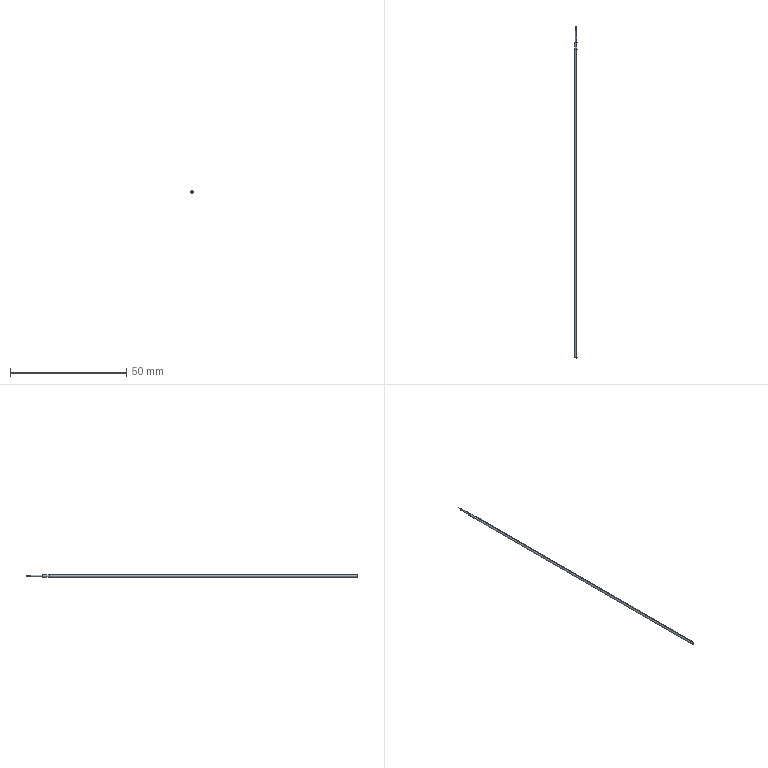Part | SolidWorks | features ICE 3, Extrusion 1 | 1 solid | 13 faces | box 1.13 x 143 x 1.13 mm | volume 137.726 mm3 | cylinder 8 | plane 5 | commonest cylinder face diameters 0.2 x2 0.7 x2 1 x2 1.13 x2
STEP:
#1=CARTESIAN_POINT('',(0.,143.,0.1));
#2=VERTEX_POINT('',#1);
#3=CARTESIAN_POINT('',(0.,143.,-0.1));
#4=VERTEX_POINT('',#3);
#5=CARTESIAN_POINT('',(0.,143.,0.));
#6=DIRECTION('',(0.,1.,0.));
#7=DIRECTION('',(0.,0.,1.));
#8=AXIS2_PLACEMENT_3D('',#5,#6,#7);
#9=CIRCLE('',#8,0.1);
#10=EDGE_CURVE('',#2,#4,#9,.T.);
#11=ORIENTED_EDGE('',*,*,#10,.F.);
#12=CARTESIAN_POINT('',(0.,141.,0.1));
#13=VERTEX_POINT('',#12);
#14=CARTESIAN_POINT('',(0.,143.,0.1));
#15=DIRECTION('',(0.,-1.,0.));
#16=VECTOR('',#15,1000.);
#17=LINE('',#14,#16);
#18=EDGE_CURVE('',#2,#13,#17,.T.);
#19=ORIENTED_EDGE('',*,*,#18,.T.);
#20=CARTESIAN_POINT('',(0.,141.,-0.1));
#21=VERTEX_POINT('',#20);
#22=CARTESIAN_POINT('',(0.,141.,0.));
#23=DIRECTION('',(0.,1.,0.));
#24=DIRECTION('',(0.,0.,1.));
#25=AXIS2_PLACEMENT_3D('',#22,#23,#24);
#26=CIRCLE('',#25,0.1);
#27=EDGE_CURVE('',#13,#21,#26,.T.);
#28=ORIENTED_EDGE('',*,*,#27,.T.);
#29=CARTESIAN_POINT('',(0.,143.,-0.1));
#30=DIRECTION('',(0.,-1.,0.));
#31=VECTOR('',#30,1000.);
#32=LINE('',#29,#31);
#33=EDGE_CURVE('',#4,#21,#32,.T.);
#34=ORIENTED_EDGE('',*,*,#33,.F.);
#35=EDGE_LOOP('',(#11,#19,#28,#34));
#36=FACE_OUTER_BOUND('',#35,.T.);
#37=CARTESIAN_POINT('',(0.,143.,0.));
#38=DIRECTION('',(0.,-1.,0.));
#39=DIRECTION('',(0.,0.,-1.));
#40=AXIS2_PLACEMENT_3D('',#37,#38,#39);
#41=CYLINDRICAL_SURFACE('',#40,0.1);
#42=ADVANCED_FACE('',(#36),#41,.T.);
#43=CARTESIAN_POINT('',(0.,141.,0.35));
#44=VERTEX_POINT('',#43);
#45=CARTESIAN_POINT('',(0.,141.,-0.35));
#46=VERTEX_POINT('',#45);
#47=CARTESIAN_POINT('',(0.,141.,0.));
#48=DIRECTION('',(0.,1.,0.));
#49=DIRECTION('',(0.,0.,1.));
#50=AXIS2_PLACEMENT_3D('',#47,#48,#49);
#51=CIRCLE('',#50,0.35);
#52=EDGE_CURVE('',#44,#46,#51,.T.);
#53=ORIENTED_EDGE('',*,*,#52,.F.);
#54=CARTESIAN_POINT('',(0.,136.,0.35));
#55=VERTEX_POINT('',#54);
#56=CARTESIAN_POINT('',(0.,141.,0.35));
#57=DIRECTION('',(0.,-1.,0.));
#58=VECTOR('',#57,1000.);
#59=LINE('',#56,#58);
#60=EDGE_CURVE('',#44,#55,#59,.T.);
#61=ORIENTED_EDGE('',*,*,#60,.T.);
#62=CARTESIAN_POINT('',(0.,136.,-0.35));
#63=VERTEX_POINT('',#62);
#64=CARTESIAN_POINT('',(0.,136.,0.));
#65=DIRECTION('',(0.,1.,0.));
#66=DIRECTION('',(0.,0.,1.));
#67=AXIS2_PLACEMENT_3D('',#64,#65,#66);
#68=CIRCLE('',#67,0.35);
#69=EDGE_CURVE('',#55,#63,#68,.T.);
#70=ORIENTED_EDGE('',*,*,#69,.T.);
#71=CARTESIAN_POINT('',(0.,141.,-0.35));
#72=DIRECTION('',(0.,-1.,0.));
#73=VECTOR('',#72,1000.);
#74=LINE('',#71,#73);
#75=EDGE_CURVE('',#46,#63,#74,.T.);
#76=ORIENTED_EDGE('',*,*,#75,.F.);
#77=EDGE_LOOP('',(#53,#61,#70,#76));
#78=FACE_OUTER_BOUND('',#77,.T.);
#79=CARTESIAN_POINT('',(0.,141.,0.));
#80=DIRECTION('',(0.,-1.,0.));
#81=DIRECTION('',(0.,0.,-1.));
#82=AXIS2_PLACEMENT_3D('',#79,#80,#81);
#83=CYLINDRICAL_SURFACE('',#82,0.35);
#84=ADVANCED_FACE('',(#78),#83,.T.);
#85=CARTESIAN_POINT('',(0.,136.,0.5));
#86=VERTEX_POINT('',#85);
#87=CARTESIAN_POINT('',(0.,136.,-0.5));
#88=VERTEX_POINT('',#87);
#89=CARTESIAN_POINT('',(0.,136.,0.));
#90=DIRECTION('',(0.,1.,0.));
#91=DIRECTION('',(0.,0.,1.));
#92=AXIS2_PLACEMENT_3D('',#89,#90,#91);
#93=CIRCLE('',#92,0.5);
#94=EDGE_CURVE('',#86,#88,#93,.T.);
#95=ORIENTED_EDGE('',*,*,#94,.F.);
#96=CARTESIAN_POINT('',(0.,133.,0.5));
#97=VERTEX_POINT('',#96);
#98=CARTESIAN_POINT('',(0.,136.,0.5));
#99=DIRECTION('',(0.,-1.,0.));
#100=VECTOR('',#99,1000.);
#101=LINE('',#98,#100);
#102=EDGE_CURVE('',#86,#97,#101,.T.);
#103=ORIENTED_EDGE('',*,*,#102,.T.);
#104=CARTESIAN_POINT('',(0.,133.,-0.5));
#105=VERTEX_POINT('',#104);
#106=CARTESIAN_POINT('',(0.,133.,0.));
#107=DIRECTION('',(0.,1.,0.));
#108=DIRECTION('',(0.,0.,1.));
#109=AXIS2_PLACEMENT_3D('',#106,#107,#108);
#110=CIRCLE('',#109,0.5);
#111=EDGE_CURVE('',#97,#105,#110,.T.);
#112=ORIENTED_EDGE('',*,*,#111,.T.);
#113=CARTESIAN_POINT('',(0.,136.,-0.5));
#114=DIRECTION('',(0.,-1.,0.));
#115=VECTOR('',#114,1000.);
#116=LINE('',#113,#115);
#117=EDGE_CURVE('',#88,#105,#116,.T.);
#118=ORIENTED_EDGE('',*,*,#117,.F.);
#119=EDGE_LOOP('',(#95,#103,#112,#118));
#120=FACE_OUTER_BOUND('',#119,.T.);
#121=CARTESIAN_POINT('',(0.,136.,0.));
#122=DIRECTION('',(0.,-1.,0.));
#123=DIRECTION('',(0.,0.,-1.));
#124=AXIS2_PLACEMENT_3D('',#121,#122,#123);
#125=CYLINDRICAL_SURFACE('',#124,0.5);
#126=ADVANCED_FACE('',(#120),#125,.T.);
#127=CARTESIAN_POINT('',(0.,133.,0.565));
#128=VERTEX_POINT('',#127);
#129=CARTESIAN_POINT('',(0.,133.,-0.565));
#130=VERTEX_POINT('',#129);
#131=CARTESIAN_POINT('',(0.,133.,0.));
#132=DIRECTION('',(0.,1.,0.));
#133=DIRECTION('',(0.,0.,1.));
#134=AXIS2_PLACEMENT_3D('',#131,#132,#133);
#135=CIRCLE('',#134,0.565);
#136=EDGE_CURVE('',#128,#130,#135,.T.);
#137=ORIENTED_EDGE('',*,*,#136,.F.);
#138=CARTESIAN_POINT('',(0.,0.,0.565));
#139=VERTEX_POINT('',#138);
#140=CARTESIAN_POINT('',(0.,133.,0.565));
#141=DIRECTION('',(0.,-1.,0.));
#142=VECTOR('',#141,1000.);
#143=LINE('',#140,#142);
#144=EDGE_CURVE('',#128,#139,#143,.T.);
#145=ORIENTED_EDGE('',*,*,#144,.T.);
#146=CARTESIAN_POINT('',(0.,0.,-0.565));
#147=VERTEX_POINT('',#146);
#148=CARTESIAN_POINT('',(0.,0.,0.));
#149=DIRECTION('',(0.,1.,0.));
#150=DIRECTION('',(0.,0.,1.));
#151=AXIS2_PLACEMENT_3D('',#148,#149,#150);
#152=CIRCLE('',#151,0.565);
#153=EDGE_CURVE('',#139,#147,#152,.T.);
#154=ORIENTED_EDGE('',*,*,#153,.T.);
#155=CARTESIAN_POINT('',(0.,133.,-0.565));
#156=DIRECTION('',(0.,-1.,0.));
#157=VECTOR('',#156,1000.);
#158=LINE('',#155,#157);
#159=EDGE_CURVE('',#130,#147,#158,.T.);
#160=ORIENTED_EDGE('',*,*,#159,.F.);
#161=EDGE_LOOP('',(#137,#145,#154,#160));
#162=FACE_OUTER_BOUND('',#161,.T.);
#163=CARTESIAN_POINT('',(0.,133.,0.));
#164=DIRECTION('',(0.,-1.,0.));
#165=DIRECTION('',(0.,0.,-1.));
#166=AXIS2_PLACEMENT_3D('',#163,#164,#165);
#167=CYLINDRICAL_SURFACE('',#166,0.565);
#168=ADVANCED_FACE('',(#162),#167,.T.);
#169=CARTESIAN_POINT('',(0.,141.,0.));
#170=DIRECTION('',(0.,1.,0.));
#171=DIRECTION('',(0.,0.,1.));
#172=AXIS2_PLACEMENT_3D('',#169,#170,#171);
#173=CIRCLE('',#172,0.35);
#174=EDGE_CURVE('',#46,#44,#173,.T.);
#175=ORIENTED_EDGE('',*,*,#174,.T.);
#176=ORIENTED_EDGE('',*,*,#52,.T.);
#177=EDGE_LOOP('',(#175,#176));
#178=FACE_OUTER_BOUND('',#177,.T.);
#179=CARTESIAN_POINT('',(0.,141.,0.));
#180=DIRECTION('',(0.,1.,0.));
#181=DIRECTION('',(0.,0.,1.));
#182=AXIS2_PLACEMENT_3D('',#179,#180,#181);
#183=CIRCLE('',#182,0.1);
#184=EDGE_CURVE('',#21,#13,#183,.T.);
#185=ORIENTED_EDGE('',*,*,#184,.F.);
#186=ORIENTED_EDGE('',*,*,#27,.F.);
#187=EDGE_LOOP('',(#185,#186));
#188=FACE_BOUND('',#187,.T.);
#189=CARTESIAN_POINT('',(0.,141.,0.));
#190=DIRECTION('',(0.,1.,0.));
#191=DIRECTION('',(0.,0.,1.));
#192=AXIS2_PLACEMENT_3D('',#189,#190,#191);
#193=PLANE('',#192);
#194=ADVANCED_FACE('',(#178,#188),#193,.T.);
#195=CARTESIAN_POINT('',(0.,136.,0.));
#196=DIRECTION('',(0.,1.,0.));
#197=DIRECTION('',(0.,0.,1.));
#198=AXIS2_PLACEMENT_3D('',#195,#196,#197);
#199=CIRCLE('',#198,0.5);
#200=EDGE_CURVE('',#88,#86,#199,.T.);
#201=ORIENTED_EDGE('',*,*,#200,.T.);
#202=ORIENTED_EDGE('',*,*,#94,.T.);
#203=EDGE_LOOP('',(#201,#202));
#204=FACE_OUTER_BOUND('',#203,.T.);
#205=CARTESIAN_POINT('',(0.,136.,0.));
#206=DIRECTION('',(0.,1.,0.));
#207=DIRECTION('',(0.,0.,1.));
#208=AXIS2_PLACEMENT_3D('',#205,#206,#207);
#209=CIRCLE('',#208,0.35);
#210=EDGE_CURVE('',#63,#55,#209,.T.);
#211=ORIENTED_EDGE('',*,*,#210,.F.);
#212=ORIENTED_EDGE('',*,*,#69,.F.);
#213=EDGE_LOOP('',(#211,#212));
#214=FACE_BOUND('',#213,.T.);
#215=CARTESIAN_POINT('',(0.,136.,0.));
#216=DIRECTION('',(0.,1.,0.));
#217=DIRECTION('',(0.,0.,1.));
#218=AXIS2_PLACEMENT_3D('',#215,#216,#217);
#219=PLANE('',#218);
#220=ADVANCED_FACE('',(#204,#214),#219,.T.);
#221=CARTESIAN_POINT('',(0.,133.,0.));
#222=DIRECTION('',(0.,1.,0.));
#223=DIRECTION('',(0.,0.,1.));
#224=AXIS2_PLACEMENT_3D('',#221,#222,#223);
#225=CIRCLE('',#224,0.565);
#226=EDGE_CURVE('',#130,#128,#225,.T.);
#227=ORIENTED_EDGE('',*,*,#226,.T.);
#228=ORIENTED_EDGE('',*,*,#136,.T.);
#229=EDGE_LOOP('',(#227,#228));
#230=FACE_OUTER_BOUND('',#229,.T.);
#231=CARTESIAN_POINT('',(0.,133.,0.));
#232=DIRECTION('',(0.,1.,0.));
#233=DIRECTION('',(0.,0.,1.));
#234=AXIS2_PLACEMENT_3D('',#231,#232,#233);
#235=CIRCLE('',#234,0.5);
#236=EDGE_CURVE('',#105,#97,#235,.T.);
#237=ORIENTED_EDGE('',*,*,#236,.F.);
#238=ORIENTED_EDGE('',*,*,#111,.F.);
#239=EDGE_LOOP('',(#237,#238));
#240=FACE_BOUND('',#239,.T.);
#241=CARTESIAN_POINT('',(0.,133.,0.));
#242=DIRECTION('',(0.,1.,0.));
#243=DIRECTION('',(0.,0.,1.));
#244=AXIS2_PLACEMENT_3D('',#241,#242,#243);
#245=PLANE('',#244);
#246=ADVANCED_FACE('',(#230,#240),#245,.T.);
#247=ORIENTED_EDGE('',*,*,#144,.F.);
#248=ORIENTED_EDGE('',*,*,#226,.F.);
#249=ORIENTED_EDGE('',*,*,#159,.T.);
#250=CARTESIAN_POINT('',(0.,0.,0.));
#251=DIRECTION('',(0.,1.,0.));
#252=DIRECTION('',(0.,0.,1.));
#253=AXIS2_PLACEMENT_3D('',#250,#251,#252);
#254=CIRCLE('',#253,0.565);
#255=EDGE_CURVE('',#147,#139,#254,.T.);
#256=ORIENTED_EDGE('',*,*,#255,.T.);
#257=EDGE_LOOP('',(#247,#248,#249,#256));
#258=FACE_OUTER_BOUND('',#257,.T.);
#259=CARTESIAN_POINT('',(0.,133.,0.));
#260=DIRECTION('',(0.,-1.,0.));
#261=DIRECTION('',(0.,0.,-1.));
#262=AXIS2_PLACEMENT_3D('',#259,#260,#261);
#263=CYLINDRICAL_SURFACE('',#262,0.565);
#264=ADVANCED_FACE('',(#258),#263,.T.);
#265=ORIENTED_EDGE('',*,*,#255,.F.);
#266=ORIENTED_EDGE('',*,*,#153,.F.);
#267=EDGE_LOOP('',(#265,#266));
#268=FACE_OUTER_BOUND('',#267,.T.);
#269=CARTESIAN_POINT('',(0.,0.,0.));
#270=DIRECTION('',(0.,1.,0.));
#271=DIRECTION('',(0.,0.,1.));
#272=AXIS2_PLACEMENT_3D('',#269,#270,#271);
#273=PLANE('',#272);
#274=ADVANCED_FACE('',(#268),#273,.F.);
#275=ORIENTED_EDGE('',*,*,#102,.F.);
#276=ORIENTED_EDGE('',*,*,#200,.F.);
#277=ORIENTED_EDGE('',*,*,#117,.T.);
#278=ORIENTED_EDGE('',*,*,#236,.T.);
#279=EDGE_LOOP('',(#275,#276,#277,#278));
#280=FACE_OUTER_BOUND('',#279,.T.);
#281=CARTESIAN_POINT('',(0.,136.,0.));
#282=DIRECTION('',(0.,-1.,0.));
#283=DIRECTION('',(0.,0.,-1.));
#284=AXIS2_PLACEMENT_3D('',#281,#282,#283);
#285=CYLINDRICAL_SURFACE('',#284,0.5);
#286=ADVANCED_FACE('',(#280),#285,.T.);
#287=ORIENTED_EDGE('',*,*,#60,.F.);
#288=ORIENTED_EDGE('',*,*,#174,.F.);
#289=ORIENTED_EDGE('',*,*,#75,.T.);
#290=ORIENTED_EDGE('',*,*,#210,.T.);
#291=EDGE_LOOP('',(#287,#288,#289,#290));
#292=FACE_OUTER_BOUND('',#291,.T.);
#293=CARTESIAN_POINT('',(0.,141.,0.));
#294=DIRECTION('',(0.,-1.,0.));
#295=DIRECTION('',(0.,0.,-1.));
#296=AXIS2_PLACEMENT_3D('',#293,#294,#295);
#297=CYLINDRICAL_SURFACE('',#296,0.35);
#298=ADVANCED_FACE('',(#292),#297,.T.);
#299=ORIENTED_EDGE('',*,*,#18,.F.);
#300=CARTESIAN_POINT('',(0.,143.,0.));
#301=DIRECTION('',(0.,1.,0.));
#302=DIRECTION('',(0.,0.,1.));
#303=AXIS2_PLACEMENT_3D('',#300,#301,#302);
#304=CIRCLE('',#303,0.1);
#305=EDGE_CURVE('',#4,#2,#304,.T.);
#306=ORIENTED_EDGE('',*,*,#305,.F.);
#307=ORIENTED_EDGE('',*,*,#33,.T.);
#308=ORIENTED_EDGE('',*,*,#184,.T.);
#309=EDGE_LOOP('',(#299,#306,#307,#308));
#310=FACE_OUTER_BOUND('',#309,.T.);
#311=CARTESIAN_POINT('',(0.,143.,0.));
#312=DIRECTION('',(0.,-1.,0.));
#313=DIRECTION('',(0.,0.,-1.));
#314=AXIS2_PLACEMENT_3D('',#311,#312,#313);
#315=CYLINDRICAL_SURFACE('',#314,0.1);
#316=ADVANCED_FACE('',(#310),#315,.T.);
#317=ORIENTED_EDGE('',*,*,#305,.T.);
#318=ORIENTED_EDGE('',*,*,#10,.T.);
#319=EDGE_LOOP('',(#317,#318));
#320=FACE_OUTER_BOUND('',#319,.T.);
#321=CARTESIAN_POINT('',(0.,143.,0.));
#322=DIRECTION('',(0.,1.,0.));
#323=DIRECTION('',(0.,0.,1.));
#324=AXIS2_PLACEMENT_3D('',#321,#322,#323);
#325=PLANE('',#324);
#326=ADVANCED_FACE('',(#320),#325,.T.);
#327=CLOSED_SHELL('',(#42,#84,#126,#168,#194,#220,#246,#264,#274,#286,#298,#316,#326));
#328=MANIFOLD_SOLID_BREP('',#327);
#329=CARTESIAN_POINT('',(0.,0.,0.));
#330=DIRECTION('',(0.,0.,1.));
#331=DIRECTION('',(1.,0.,0.));
#332=AXIS2_PLACEMENT_3D('',#329,#330,#331);
#333=(LENGTH_UNIT()NAMED_UNIT(*)SI_UNIT(.MILLI.,.METRE.));
#334=UNCERTAINTY_MEASURE_WITH_UNIT(LENGTH_MEASURE(0.00001),#333,'','');
#335=(NAMED_UNIT(*)PLANE_ANGLE_UNIT()SI_UNIT($,.RADIAN.));
#336=(NAMED_UNIT(*)SI_UNIT($,.STERADIAN.)SOLID_ANGLE_UNIT());
#337=(GEOMETRIC_REPRESENTATION_CONTEXT(3)GLOBAL_UNCERTAINTY_ASSIGNED_CONTEXT((#334))GLOBAL_UNIT_ASSIGNED_CONTEXT((#333,#335,#336))REPRESENTATION_CONTEXT('',''));
#338=ADVANCED_BREP_SHAPE_REPRESENTATION('',(#328,#332),#337);